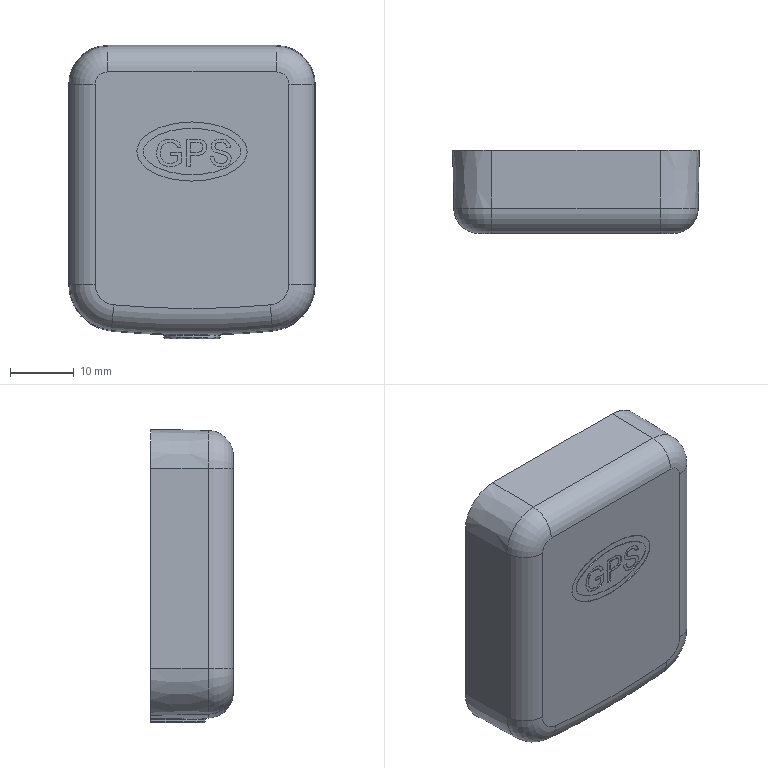Part | SolidWorks | features ICE 11, Fillet 4, Extrusion 1, RevCut 1 | 1 solid | 217 faces | box 38.7 x 13 x 46 mm | volume 6467 mm3 | plane 86 | cylinder 61 | spline 44 | torus 14 | cone 12 | commonest cylinder face diameters 1.65 x18 4 x13 1.5 x8 4.2 x4 8 x3 10.4 x3